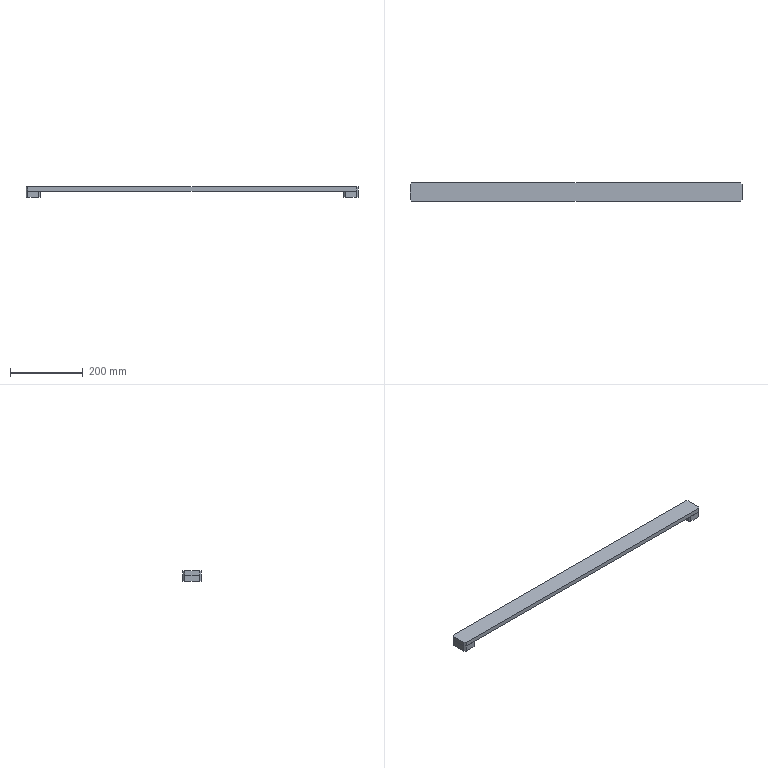Part | SolidWorks | features BaseBody 3 | 3 solids | 30 faces | box 913 x 50 x 29 mm | volume 613500 mm3 | plane 30
STEP:
#1=CARTESIAN_POINT('',(456.5,-20.,12.));
#2=VERTEX_POINT('',#1);
#3=CARTESIAN_POINT('',(456.5,20.,12.));
#4=VERTEX_POINT('',#3);
#5=CARTESIAN_POINT('',(456.5,25.,12.));
#6=DIRECTION('',(0.,1.,0.));
#7=VECTOR('',#6,1000.);
#8=LINE('',#5,#7);
#9=EDGE_CURVE('',#2,#4,#8,.T.);
#10=ORIENTED_EDGE('',*,*,#9,.F.);
#11=CARTESIAN_POINT('',(456.5,-20.,0.));
#12=VERTEX_POINT('',#11);
#13=CARTESIAN_POINT('',(456.5,-20.,12.));
#14=DIRECTION('',(0.,0.,-1.));
#15=VECTOR('',#14,1000.);
#16=LINE('',#13,#15);
#17=EDGE_CURVE('',#2,#12,#16,.T.);
#18=ORIENTED_EDGE('',*,*,#17,.T.);
#19=CARTESIAN_POINT('',(456.5,20.,0.));
#20=VERTEX_POINT('',#19);
#21=CARTESIAN_POINT('',(456.5,25.,0.));
#22=DIRECTION('',(0.,1.,0.));
#23=VECTOR('',#22,1000.);
#24=LINE('',#21,#23);
#25=EDGE_CURVE('',#12,#20,#24,.T.);
#26=ORIENTED_EDGE('',*,*,#25,.T.);
#27=CARTESIAN_POINT('',(456.5,20.,12.));
#28=DIRECTION('',(0.,0.,1.));
#29=VECTOR('',#28,1000.);
#30=LINE('',#27,#29);
#31=EDGE_CURVE('',#20,#4,#30,.T.);
#32=ORIENTED_EDGE('',*,*,#31,.T.);
#33=EDGE_LOOP('',(#10,#18,#26,#32));
#34=FACE_OUTER_BOUND('',#33,.T.);
#35=CARTESIAN_POINT('',(456.5,25.,12.));
#36=DIRECTION('',(-1.,0.,0.));
#37=DIRECTION('',(0.,0.,1.));
#38=AXIS2_PLACEMENT_3D('',#35,#36,#37);
#39=PLANE('',#38);
#40=ADVANCED_FACE('',(#34),#39,.F.);
#41=CARTESIAN_POINT('',(451.5,25.,0.));
#42=VERTEX_POINT('',#41);
#43=CARTESIAN_POINT('',(-451.5,25.,0.));
#44=VERTEX_POINT('',#43);
#45=CARTESIAN_POINT('',(-456.5,25.,0.));
#46=DIRECTION('',(-1.,0.,0.));
#47=VECTOR('',#46,1000.);
#48=LINE('',#45,#47);
#49=EDGE_CURVE('',#42,#44,#48,.T.);
#50=ORIENTED_EDGE('',*,*,#49,.T.);
#51=CARTESIAN_POINT('',(-451.5,25.,12.));
#52=VERTEX_POINT('',#51);
#53=CARTESIAN_POINT('',(-451.5,25.,12.));
#54=DIRECTION('',(0.,0.,1.));
#55=VECTOR('',#54,1000.);
#56=LINE('',#53,#55);
#57=EDGE_CURVE('',#44,#52,#56,.T.);
#58=ORIENTED_EDGE('',*,*,#57,.T.);
#59=CARTESIAN_POINT('',(451.5,25.,12.));
#60=VERTEX_POINT('',#59);
#61=CARTESIAN_POINT('',(-130.,25.,12.));
#62=DIRECTION('',(-1.,0.,0.));
#63=VECTOR('',#62,1000.);
#64=LINE('',#61,#63);
#65=EDGE_CURVE('',#60,#52,#64,.T.);
#66=ORIENTED_EDGE('',*,*,#65,.F.);
#67=CARTESIAN_POINT('',(451.5,25.,12.));
#68=DIRECTION('',(0.,0.,-1.));
#69=VECTOR('',#68,1000.);
#70=LINE('',#67,#69);
#71=EDGE_CURVE('',#60,#42,#70,.T.);
#72=ORIENTED_EDGE('',*,*,#71,.T.);
#73=EDGE_LOOP('',(#50,#58,#66,#72));
#74=FACE_OUTER_BOUND('',#73,.T.);
#75=CARTESIAN_POINT('',(-456.5,25.,12.));
#76=DIRECTION('',(0.,-1.,0.));
#77=DIRECTION('',(0.,0.,-1.));
#78=AXIS2_PLACEMENT_3D('',#75,#76,#77);
#79=PLANE('',#78);
#80=ADVANCED_FACE('',(#74),#79,.F.);
#81=CARTESIAN_POINT('',(-456.5,20.,12.));
#82=VERTEX_POINT('',#81);
#83=CARTESIAN_POINT('',(-456.5,-20.,12.));
#84=VERTEX_POINT('',#83);
#85=CARTESIAN_POINT('',(-456.5,25.,12.));
#86=DIRECTION('',(0.,-1.,0.));
#87=VECTOR('',#86,1000.);
#88=LINE('',#85,#87);
#89=EDGE_CURVE('',#82,#84,#88,.T.);
#90=ORIENTED_EDGE('',*,*,#89,.F.);
#91=CARTESIAN_POINT('',(-456.5,20.,0.));
#92=VERTEX_POINT('',#91);
#93=CARTESIAN_POINT('',(-456.5,20.,12.));
#94=DIRECTION('',(0.,0.,-1.));
#95=VECTOR('',#94,1000.);
#96=LINE('',#93,#95);
#97=EDGE_CURVE('',#82,#92,#96,.T.);
#98=ORIENTED_EDGE('',*,*,#97,.T.);
#99=CARTESIAN_POINT('',(-456.5,-20.,0.));
#100=VERTEX_POINT('',#99);
#101=CARTESIAN_POINT('',(-456.5,25.,0.));
#102=DIRECTION('',(0.,-1.,0.));
#103=VECTOR('',#102,1000.);
#104=LINE('',#101,#103);
#105=EDGE_CURVE('',#92,#100,#104,.T.);
#106=ORIENTED_EDGE('',*,*,#105,.T.);
#107=CARTESIAN_POINT('',(-456.5,-20.,12.));
#108=DIRECTION('',(0.,0.,1.));
#109=VECTOR('',#108,1000.);
#110=LINE('',#107,#109);
#111=EDGE_CURVE('',#100,#84,#110,.T.);
#112=ORIENTED_EDGE('',*,*,#111,.T.);
#113=EDGE_LOOP('',(#90,#98,#106,#112));
#114=FACE_OUTER_BOUND('',#113,.T.);
#115=CARTESIAN_POINT('',(-456.5,25.,12.));
#116=DIRECTION('',(1.,0.,0.));
#117=DIRECTION('',(0.,0.,-1.));
#118=AXIS2_PLACEMENT_3D('',#115,#116,#117);
#119=PLANE('',#118);
#120=ADVANCED_FACE('',(#114),#119,.F.);
#121=CARTESIAN_POINT('',(-451.5,-25.,12.));
#122=VERTEX_POINT('',#121);
#123=CARTESIAN_POINT('',(451.5,-25.,12.));
#124=VERTEX_POINT('',#123);
#125=CARTESIAN_POINT('',(-456.5,-25.,12.));
#126=DIRECTION('',(1.,0.,0.));
#127=VECTOR('',#126,1000.);
#128=LINE('',#125,#127);
#129=EDGE_CURVE('',#122,#124,#128,.T.);
#130=ORIENTED_EDGE('',*,*,#129,.F.);
#131=CARTESIAN_POINT('',(-451.5,-25.,0.));
#132=VERTEX_POINT('',#131);
#133=CARTESIAN_POINT('',(-451.5,-25.,12.));
#134=DIRECTION('',(0.,0.,-1.));
#135=VECTOR('',#134,1000.);
#136=LINE('',#133,#135);
#137=EDGE_CURVE('',#122,#132,#136,.T.);
#138=ORIENTED_EDGE('',*,*,#137,.T.);
#139=CARTESIAN_POINT('',(451.5,-25.,0.));
#140=VERTEX_POINT('',#139);
#141=CARTESIAN_POINT('',(-456.5,-25.,0.));
#142=DIRECTION('',(1.,0.,0.));
#143=VECTOR('',#142,1000.);
#144=LINE('',#141,#143);
#145=EDGE_CURVE('',#132,#140,#144,.T.);
#146=ORIENTED_EDGE('',*,*,#145,.T.);
#147=CARTESIAN_POINT('',(451.5,-25.,12.));
#148=DIRECTION('',(0.,0.,1.));
#149=VECTOR('',#148,1000.);
#150=LINE('',#147,#149);
#151=EDGE_CURVE('',#140,#124,#150,.T.);
#152=ORIENTED_EDGE('',*,*,#151,.T.);
#153=EDGE_LOOP('',(#130,#138,#146,#152));
#154=FACE_OUTER_BOUND('',#153,.T.);
#155=CARTESIAN_POINT('',(-456.5,-25.,12.));
#156=DIRECTION('',(0.,1.,0.));
#157=DIRECTION('',(0.,0.,1.));
#158=AXIS2_PLACEMENT_3D('',#155,#156,#157);
#159=PLANE('',#158);
#160=ADVANCED_FACE('',(#154),#159,.F.);
#161=ORIENTED_EDGE('',*,*,#65,.T.);
#162=CARTESIAN_POINT('',(-238.25,238.25,12.));
#163=DIRECTION('',(-0.7071,-0.7071,0.));
#164=VECTOR('',#163,1000.);
#165=LINE('',#162,#164);
#166=EDGE_CURVE('',#52,#82,#165,.T.);
#167=ORIENTED_EDGE('',*,*,#166,.T.);
#168=ORIENTED_EDGE('',*,*,#89,.T.);
#169=CARTESIAN_POINT('',(-238.25,-238.25,12.));
#170=DIRECTION('',(0.7071,-0.7071,0.));
#171=VECTOR('',#170,1000.);
#172=LINE('',#169,#171);
#173=EDGE_CURVE('',#84,#122,#172,.T.);
#174=ORIENTED_EDGE('',*,*,#173,.T.);
#175=ORIENTED_EDGE('',*,*,#129,.T.);
#176=CARTESIAN_POINT('',(238.25,-238.25,12.));
#177=DIRECTION('',(0.7071,0.7071,0.));
#178=VECTOR('',#177,1000.);
#179=LINE('',#176,#178);
#180=EDGE_CURVE('',#124,#2,#179,.T.);
#181=ORIENTED_EDGE('',*,*,#180,.T.);
#182=ORIENTED_EDGE('',*,*,#9,.T.);
#183=CARTESIAN_POINT('',(238.25,238.25,12.));
#184=DIRECTION('',(-0.7071,0.7071,0.));
#185=VECTOR('',#184,1000.);
#186=LINE('',#183,#185);
#187=EDGE_CURVE('',#4,#60,#186,.T.);
#188=ORIENTED_EDGE('',*,*,#187,.T.);
#189=EDGE_LOOP('',(#161,#167,#168,#174,#175,#181,#182,#188));
#190=FACE_OUTER_BOUND('',#189,.T.);
#191=CARTESIAN_POINT('',(0.,0.,12.));
#192=DIRECTION('',(0.,0.,1.));
#193=DIRECTION('',(1.,0.,0.));
#194=AXIS2_PLACEMENT_3D('',#191,#192,#193);
#195=PLANE('',#194);
#196=ADVANCED_FACE('',(#190),#195,.T.);
#197=ORIENTED_EDGE('',*,*,#105,.F.);
#198=CARTESIAN_POINT('',(-456.5,20.,0.));
#199=DIRECTION('',(0.7071,0.7071,0.));
#200=VECTOR('',#199,1000.);
#201=LINE('',#198,#200);
#202=EDGE_CURVE('',#92,#44,#201,.T.);
#203=ORIENTED_EDGE('',*,*,#202,.T.);
#204=ORIENTED_EDGE('',*,*,#49,.F.);
#205=CARTESIAN_POINT('',(451.5,25.,0.));
#206=DIRECTION('',(0.7071,-0.7071,0.));
#207=VECTOR('',#206,1000.);
#208=LINE('',#205,#207);
#209=EDGE_CURVE('',#42,#20,#208,.T.);
#210=ORIENTED_EDGE('',*,*,#209,.T.);
#211=ORIENTED_EDGE('',*,*,#25,.F.);
#212=CARTESIAN_POINT('',(456.5,-20.,0.));
#213=DIRECTION('',(-0.7071,-0.7071,0.));
#214=VECTOR('',#213,1000.);
#215=LINE('',#212,#214);
#216=EDGE_CURVE('',#12,#140,#215,.T.);
#217=ORIENTED_EDGE('',*,*,#216,.T.);
#218=ORIENTED_EDGE('',*,*,#145,.F.);
#219=CARTESIAN_POINT('',(-451.5,-25.,0.));
#220=DIRECTION('',(-0.7071,0.7071,0.));
#221=VECTOR('',#220,1000.);
#222=LINE('',#219,#221);
#223=EDGE_CURVE('',#132,#100,#222,.T.);
#224=ORIENTED_EDGE('',*,*,#223,.T.);
#225=EDGE_LOOP('',(#197,#203,#204,#210,#211,#217,#218,#224));
#226=FACE_OUTER_BOUND('',#225,.T.);
#227=CARTESIAN_POINT('',(0.,0.,0.));
#228=DIRECTION('',(0.,0.,1.));
#229=DIRECTION('',(1.,0.,0.));
#230=AXIS2_PLACEMENT_3D('',#227,#228,#229);
#231=PLANE('',#230);
#232=ADVANCED_FACE('',(#226),#231,.F.);
#233=ORIENTED_EDGE('',*,*,#166,.F.);
#234=ORIENTED_EDGE('',*,*,#57,.F.);
#235=ORIENTED_EDGE('',*,*,#202,.F.);
#236=ORIENTED_EDGE('',*,*,#97,.F.);
#237=EDGE_LOOP('',(#233,#234,#235,#236));
#238=FACE_OUTER_BOUND('',#237,.T.);
#239=CARTESIAN_POINT('',(-456.5,20.,12.));
#240=DIRECTION('',(0.7071,-0.7071,0.));
#241=DIRECTION('',(0.,0.,-1.));
#242=AXIS2_PLACEMENT_3D('',#239,#240,#241);
#243=PLANE('',#242);
#244=ADVANCED_FACE('',(#238),#243,.F.);
#245=ORIENTED_EDGE('',*,*,#173,.F.);
#246=ORIENTED_EDGE('',*,*,#111,.F.);
#247=ORIENTED_EDGE('',*,*,#223,.F.);
#248=ORIENTED_EDGE('',*,*,#137,.F.);
#249=EDGE_LOOP('',(#245,#246,#247,#248));
#250=FACE_OUTER_BOUND('',#249,.T.);
#251=CARTESIAN_POINT('',(-451.5,-25.,12.));
#252=DIRECTION('',(0.7071,0.7071,0.));
#253=DIRECTION('',(0.,0.,-1.));
#254=AXIS2_PLACEMENT_3D('',#251,#252,#253);
#255=PLANE('',#254);
#256=ADVANCED_FACE('',(#250),#255,.F.);
#257=ORIENTED_EDGE('',*,*,#180,.F.);
#258=ORIENTED_EDGE('',*,*,#151,.F.);
#259=ORIENTED_EDGE('',*,*,#216,.F.);
#260=ORIENTED_EDGE('',*,*,#17,.F.);
#261=EDGE_LOOP('',(#257,#258,#259,#260));
#262=FACE_OUTER_BOUND('',#261,.T.);
#263=CARTESIAN_POINT('',(456.5,-20.,12.));
#264=DIRECTION('',(-0.7071,0.7071,0.));
#265=DIRECTION('',(0.,0.,-1.));
#266=AXIS2_PLACEMENT_3D('',#263,#264,#265);
#267=PLANE('',#266);
#268=ADVANCED_FACE('',(#262),#267,.F.);
#269=ORIENTED_EDGE('',*,*,#187,.F.);
#270=ORIENTED_EDGE('',*,*,#31,.F.);
#271=ORIENTED_EDGE('',*,*,#209,.F.);
#272=ORIENTED_EDGE('',*,*,#71,.F.);
#273=EDGE_LOOP('',(#269,#270,#271,#272));
#274=FACE_OUTER_BOUND('',#273,.T.);
#275=CARTESIAN_POINT('',(451.5,25.,12.));
#276=DIRECTION('',(-0.7071,-0.7071,0.));
#277=DIRECTION('',(0.,0.,-1.));
#278=AXIS2_PLACEMENT_3D('',#275,#276,#277);
#279=PLANE('',#278);
#280=ADVANCED_FACE('',(#274),#279,.F.);
#281=CLOSED_SHELL('',(#40,#80,#120,#160,#196,#232,#244,#256,#268,#280));
#282=MANIFOLD_SOLID_BREP('',#281);
#283=CARTESIAN_POINT('',(-456.5,-20.,0.));
#284=VERTEX_POINT('',#283);
#285=CARTESIAN_POINT('',(-451.5,-25.,0.));
#286=VERTEX_POINT('',#285);
#287=CARTESIAN_POINT('',(-456.5,-20.,0.));
#288=DIRECTION('',(0.7071,-0.7071,0.));
#289=VECTOR('',#288,1000.);
#290=LINE('',#287,#289);
#291=EDGE_CURVE('',#284,#286,#290,.T.);
#292=ORIENTED_EDGE('',*,*,#291,.F.);
#293=CARTESIAN_POINT('',(-456.5,-20.,-17.));
#294=VERTEX_POINT('',#293);
#295=CARTESIAN_POINT('',(-456.5,-20.,-17.));
#296=DIRECTION('',(0.,0.,1.));
#297=VECTOR('',#296,1000.);
#298=LINE('',#295,#297);
#299=EDGE_CURVE('',#294,#284,#298,.T.);
#300=ORIENTED_EDGE('',*,*,#299,.F.);
#301=CARTESIAN_POINT('',(-451.5,-25.,-17.));
#302=VERTEX_POINT('',#301);
#303=CARTESIAN_POINT('',(-456.5,-20.,-17.));
#304=DIRECTION('',(0.7071,-0.7071,0.));
#305=VECTOR('',#304,1000.);
#306=LINE('',#303,#305);
#307=EDGE_CURVE('',#294,#302,#306,.T.);
#308=ORIENTED_EDGE('',*,*,#307,.T.);
#309=CARTESIAN_POINT('',(-451.5,-25.,-17.));
#310=DIRECTION('',(0.,0.,1.));
#311=VECTOR('',#310,1000.);
#312=LINE('',#309,#311);
#313=EDGE_CURVE('',#302,#286,#312,.T.);
#314=ORIENTED_EDGE('',*,*,#313,.T.);
#315=EDGE_LOOP('',(#292,#300,#308,#314));
#316=FACE_OUTER_BOUND('',#315,.T.);
#317=CARTESIAN_POINT('',(-456.5,-20.,-17.));
#318=DIRECTION('',(-0.7071,-0.7071,0.));
#319=DIRECTION('',(0.7071,-0.7071,0.));
#320=AXIS2_PLACEMENT_3D('',#317,#318,#319);
#321=PLANE('',#320);
#322=ADVANCED_FACE('',(#316),#321,.T.);
#323=CARTESIAN_POINT('',(-456.5,20.,0.));
#324=VERTEX_POINT('',#323);
#325=CARTESIAN_POINT('',(-456.5,-20.,0.));
#326=DIRECTION('',(0.,-1.,0.));
#327=VECTOR('',#326,1000.);
#328=LINE('',#325,#327);
#329=EDGE_CURVE('',#324,#284,#328,.T.);
#330=ORIENTED_EDGE('',*,*,#329,.F.);
#331=CARTESIAN_POINT('',(-456.5,20.,-17.));
#332=VERTEX_POINT('',#331);
#333=CARTESIAN_POINT('',(-456.5,20.,-17.));
#334=DIRECTION('',(0.,0.,1.));
#335=VECTOR('',#334,1000.);
#336=LINE('',#333,#335);
#337=EDGE_CURVE('',#332,#324,#336,.T.);
#338=ORIENTED_EDGE('',*,*,#337,.F.);
#339=CARTESIAN_POINT('',(-456.5,-20.,-17.));
#340=DIRECTION('',(0.,-1.,0.));
#341=VECTOR('',#340,1000.);
#342=LINE('',#339,#341);
#343=EDGE_CURVE('',#332,#294,#342,.T.);
#344=ORIENTED_EDGE('',*,*,#343,.T.);
#345=ORIENTED_EDGE('',*,*,#299,.T.);
#346=EDGE_LOOP('',(#330,#338,#344,#345));
#347=FACE_OUTER_BOUND('',#346,.T.);
#348=CARTESIAN_POINT('',(-456.5,-20.,-17.));
#349=DIRECTION('',(-1.,0.,0.));
#350=DIRECTION('',(0.,0.,1.));
#351=AXIS2_PLACEMENT_3D('',#348,#349,#350);
#352=PLANE('',#351);
#353=ADVANCED_FACE('',(#347),#352,.T.);
#354=CARTESIAN_POINT('',(-451.5,25.,0.));
#355=VERTEX_POINT('',#354);
#356=CARTESIAN_POINT('',(-456.5,20.,0.));
#357=DIRECTION('',(-0.7071,-0.7071,0.));
#358=VECTOR('',#357,1000.);
#359=LINE('',#356,#358);
#360=EDGE_CURVE('',#355,#324,#359,.T.);
#361=ORIENTED_EDGE('',*,*,#360,.F.);
#362=CARTESIAN_POINT('',(-451.5,25.,-17.));
#363=VERTEX_POINT('',#362);
#364=CARTESIAN_POINT('',(-451.5,25.,-17.));
#365=DIRECTION('',(0.,0.,1.));
#366=VECTOR('',#365,1000.);
#367=LINE('',#364,#366);
#368=EDGE_CURVE('',#363,#355,#367,.T.);
#369=ORIENTED_EDGE('',*,*,#368,.F.);
#370=CARTESIAN_POINT('',(-456.5,20.,-17.));
#371=DIRECTION('',(-0.7071,-0.7071,0.));
#372=VECTOR('',#371,1000.);
#373=LINE('',#370,#372);
#374=EDGE_CURVE('',#363,#332,#373,.T.);
#375=ORIENTED_EDGE('',*,*,#374,.T.);
#376=ORIENTED_EDGE('',*,*,#337,.T.);
#377=EDGE_LOOP('',(#361,#369,#375,#376));
#378=FACE_OUTER_BOUND('',#377,.T.);
#379=CARTESIAN_POINT('',(-456.5,20.,-17.));
#380=DIRECTION('',(-0.7071,0.7071,0.));
#381=DIRECTION('',(-0.7071,-0.7071,0.));
#382=AXIS2_PLACEMENT_3D('',#379,#380,#381);
#383=PLANE('',#382);
#384=ADVANCED_FACE('',(#378),#383,.T.);
#385=CARTESIAN_POINT('',(-421.5,25.,0.));
#386=VERTEX_POINT('',#385);
#387=CARTESIAN_POINT('',(-451.5,25.,0.));
#388=DIRECTION('',(-1.,0.,0.));
#389=VECTOR('',#388,1000.);
#390=LINE('',#387,#389);
#391=EDGE_CURVE('',#386,#355,#390,.T.);
#392=ORIENTED_EDGE('',*,*,#391,.F.);
#393=CARTESIAN_POINT('',(-421.5,25.,-17.));
#394=VERTEX_POINT('',#393);
#395=CARTESIAN_POINT('',(-421.5,25.,-17.));
#396=DIRECTION('',(0.,0.,1.));
#397=VECTOR('',#396,1000.);
#398=LINE('',#395,#397);
#399=EDGE_CURVE('',#394,#386,#398,.T.);
#400=ORIENTED_EDGE('',*,*,#399,.F.);
#401=CARTESIAN_POINT('',(-451.5,25.,-17.));
#402=DIRECTION('',(-1.,0.,0.));
#403=VECTOR('',#402,1000.);
#404=LINE('',#401,#403);
#405=EDGE_CURVE('',#394,#363,#404,.T.);
#406=ORIENTED_EDGE('',*,*,#405,.T.);
#407=ORIENTED_EDGE('',*,*,#368,.T.);
#408=EDGE_LOOP('',(#392,#400,#406,#407));
#409=FACE_OUTER_BOUND('',#408,.T.);
#410=CARTESIAN_POINT('',(-451.5,25.,-17.));
#411=DIRECTION('',(0.,1.,0.));
#412=DIRECTION('',(0.,0.,1.));
#413=AXIS2_PLACEMENT_3D('',#410,#411,#412);
#414=PLANE('',#413);
#415=ADVANCED_FACE('',(#409),#414,.T.);
#416=CARTESIAN_POINT('',(-416.5,20.,0.));
#417=VERTEX_POINT('',#416);
#418=CARTESIAN_POINT('',(-421.5,25.,0.));
#419=DIRECTION('',(-0.7071,0.7071,0.));
#420=VECTOR('',#419,1000.);
#421=LINE('',#418,#420);
#422=EDGE_CURVE('',#417,#386,#421,.T.);
#423=ORIENTED_EDGE('',*,*,#422,.F.);
#424=CARTESIAN_POINT('',(-416.5,20.,-17.));
#425=VERTEX_POINT('',#424);
#426=CARTESIAN_POINT('',(-416.5,20.,-17.));
#427=DIRECTION('',(0.,0.,1.));
#428=VECTOR('',#427,1000.);
#429=LINE('',#426,#428);
#430=EDGE_CURVE('',#425,#417,#429,.T.);
#431=ORIENTED_EDGE('',*,*,#430,.F.);
#432=CARTESIAN_POINT('',(-421.5,25.,-17.));
#433=DIRECTION('',(-0.7071,0.7071,0.));
#434=VECTOR('',#433,1000.);
#435=LINE('',#432,#434);
#436=EDGE_CURVE('',#425,#394,#435,.T.);
#437=ORIENTED_EDGE('',*,*,#436,.T.);
#438=ORIENTED_EDGE('',*,*,#399,.T.);
#439=EDGE_LOOP('',(#423,#431,#437,#438));
#440=FACE_OUTER_BOUND('',#439,.T.);
#441=CARTESIAN_POINT('',(-421.5,25.,-17.));
#442=DIRECTION('',(0.7071,0.7071,0.));
#443=DIRECTION('',(-0.7071,0.7071,0.));
#444=AXIS2_PLACEMENT_3D('',#441,#442,#443);
#445=PLANE('',#444);
#446=ADVANCED_FACE('',(#440),#445,.T.);
#447=CARTESIAN_POINT('',(-416.5,-20.,0.));
#448=VERTEX_POINT('',#447);
#449=CARTESIAN_POINT('',(-416.5,-20.,0.));
#450=DIRECTION('',(0.,1.,0.));
#451=VECTOR('',#450,1000.);
#452=LINE('',#449,#451);
#453=EDGE_CURVE('',#448,#417,#452,.T.);
#454=ORIENTED_EDGE('',*,*,#453,.F.);
#455=CARTESIAN_POINT('',(-416.5,-20.,-17.));
#456=VERTEX_POINT('',#455);
#457=CARTESIAN_POINT('',(-416.5,-20.,-17.));
#458=DIRECTION('',(0.,0.,1.));
#459=VECTOR('',#458,1000.);
#460=LINE('',#457,#459);
#461=EDGE_CURVE('',#456,#448,#460,.T.);
#462=ORIENTED_EDGE('',*,*,#461,.F.);
#463=CARTESIAN_POINT('',(-416.5,-20.,-17.));
#464=DIRECTION('',(0.,1.,0.));
#465=VECTOR('',#464,1000.);
#466=LINE('',#463,#465);
#467=EDGE_CURVE('',#456,#425,#466,.T.);
#468=ORIENTED_EDGE('',*,*,#467,.T.);
#469=ORIENTED_EDGE('',*,*,#430,.T.);
#470=EDGE_LOOP('',(#454,#462,#468,#469));
#471=FACE_OUTER_BOUND('',#470,.T.);
#472=CARTESIAN_POINT('',(-416.5,-20.,-17.));
#473=DIRECTION('',(1.,0.,0.));
#474=DIRECTION('',(0.,0.,-1.));
#475=AXIS2_PLACEMENT_3D('',#472,#473,#474);
#476=PLANE('',#475);
#477=ADVANCED_FACE('',(#471),#476,.T.);
#478=CARTESIAN_POINT('',(-421.5,-25.,0.));
#479=VERTEX_POINT('',#478);
#480=CARTESIAN_POINT('',(-421.5,-25.,0.));
#481=DIRECTION('',(0.7071,0.7071,0.));
#482=VECTOR('',#481,1000.);
#483=LINE('',#480,#482);
#484=EDGE_CURVE('',#479,#448,#483,.T.);
#485=ORIENTED_EDGE('',*,*,#484,.F.);
#486=CARTESIAN_POINT('',(-421.5,-25.,-17.));
#487=VERTEX_POINT('',#486);
#488=CARTESIAN_POINT('',(-421.5,-25.,-17.));
#489=DIRECTION('',(0.,0.,1.));
#490=VECTOR('',#489,1000.);
#491=LINE('',#488,#490);
#492=EDGE_CURVE('',#487,#479,#491,.T.);
#493=ORIENTED_EDGE('',*,*,#492,.F.);
#494=CARTESIAN_POINT('',(-421.5,-25.,-17.));
#495=DIRECTION('',(0.7071,0.7071,0.));
#496=VECTOR('',#495,1000.);
#497=LINE('',#494,#496);
#498=EDGE_CURVE('',#487,#456,#497,.T.);
#499=ORIENTED_EDGE('',*,*,#498,.T.);
#500=ORIENTED_EDGE('',*,*,#461,.T.);
#501=EDGE_LOOP('',(#485,#493,#499,#500));
#502=FACE_OUTER_BOUND('',#501,.T.);
#503=CARTESIAN_POINT('',(-421.5,-25.,-17.));
#504=DIRECTION('',(0.7071,-0.7071,0.));
#505=DIRECTION('',(0.7071,0.7071,0.));
#506=AXIS2_PLACEMENT_3D('',#503,#504,#505);
#507=PLANE('',#506);
#508=ADVANCED_FACE('',(#502),#507,.T.);
#509=CARTESIAN_POINT('',(-451.5,-25.,0.));
#510=DIRECTION('',(1.,0.,0.));
#511=VECTOR('',#510,1000.);
#512=LINE('',#509,#511);
#513=EDGE_CURVE('',#286,#479,#512,.T.);
#514=ORIENTED_EDGE('',*,*,#513,.F.);
#515=ORIENTED_EDGE('',*,*,#313,.F.);
#516=CARTESIAN_POINT('',(-451.5,-25.,-17.));
#517=DIRECTION('',(1.,0.,0.));
#518=VECTOR('',#517,1000.);
#519=LINE('',#516,#518);
#520=EDGE_CURVE('',#302,#487,#519,.T.);
#521=ORIENTED_EDGE('',*,*,#520,.T.);
#522=ORIENTED_EDGE('',*,*,#492,.T.);
#523=EDGE_LOOP('',(#514,#515,#521,#522));
#524=FACE_OUTER_BOUND('',#523,.T.);
#525=CARTESIAN_POINT('',(-451.5,-25.,-17.));
#526=DIRECTION('',(0.,-1.,0.));
#527=DIRECTION('',(0.,0.,-1.));
#528=AXIS2_PLACEMENT_3D('',#525,#526,#527);
#529=PLANE('',#528);
#530=ADVANCED_FACE('',(#524),#529,.T.);
#531=ORIENTED_EDGE('',*,*,#307,.F.);
#532=ORIENTED_EDGE('',*,*,#343,.F.);
#533=ORIENTED_EDGE('',*,*,#374,.F.);
#534=ORIENTED_EDGE('',*,*,#405,.F.);
#535=ORIENTED_EDGE('',*,*,#436,.F.);
#536=ORIENTED_EDGE('',*,*,#467,.F.);
#537=ORIENTED_EDGE('',*,*,#498,.F.);
#538=ORIENTED_EDGE('',*,*,#520,.F.);
#539=EDGE_LOOP('',(#531,#532,#533,#534,#535,#536,#537,#538));
#540=FACE_OUTER_BOUND('',#539,.T.);
#541=CARTESIAN_POINT('',(0.,0.,-17.));
#542=DIRECTION('',(0.,0.,1.));
#543=DIRECTION('',(1.,0.,0.));
#544=AXIS2_PLACEMENT_3D('',#541,#542,#543);
#545=PLANE('',#544);
#546=ADVANCED_FACE('',(#540),#545,.F.);
#547=ORIENTED_EDGE('',*,*,#291,.T.);
#548=ORIENTED_EDGE('',*,*,#513,.T.);
#549=ORIENTED_EDGE('',*,*,#484,.T.);
#550=ORIENTED_EDGE('',*,*,#453,.T.);
#551=ORIENTED_EDGE('',*,*,#422,.T.);
#552=ORIENTED_EDGE('',*,*,#391,.T.);
#553=ORIENTED_EDGE('',*,*,#360,.T.);
#554=ORIENTED_EDGE('',*,*,#329,.T.);
#555=EDGE_LOOP('',(#547,#548,#549,#550,#551,#552,#553,#554));
#556=FACE_OUTER_BOUND('',#555,.T.);
#557=CARTESIAN_POINT('',(0.,0.,0.));
#558=DIRECTION('',(0.,0.,1.));
#559=DIRECTION('',(1.,0.,0.));
#560=AXIS2_PLACEMENT_3D('',#557,#558,#559);
#561=PLANE('',#560);
#562=ADVANCED_FACE('',(#556),#561,.T.);
#563=CLOSED_SHELL('',(#322,#353,#384,#415,#446,#477,#508,#530,#546,#562));
#564=MANIFOLD_SOLID_BREP('',#563);
#565=CARTESIAN_POINT('',(456.5,20.,0.));
#566=VERTEX_POINT('',#565);
#567=CARTESIAN_POINT('',(451.5,25.,0.));
#568=VERTEX_POINT('',#567);
#569=CARTESIAN_POINT('',(456.5,20.,0.));
#570=DIRECTION('',(-0.7071,0.7071,0.));
#571=VECTOR('',#570,1000.);
#572=LINE('',#569,#571);
#573=EDGE_CURVE('',#566,#568,#572,.T.);
#574=ORIENTED_EDGE('',*,*,#573,.F.);
#575=CARTESIAN_POINT('',(456.5,20.,-17.));
#576=VERTEX_POINT('',#575);
#577=CARTESIAN_POINT('',(456.5,20.,-17.));
#578=DIRECTION('',(0.,0.,1.));
#579=VECTOR('',#578,1000.);
#580=LINE('',#577,#579);
#581=EDGE_CURVE('',#576,#566,#580,.T.);
#582=ORIENTED_EDGE('',*,*,#581,.F.);
#583=CARTESIAN_POINT('',(451.5,25.,-17.));
#584=VERTEX_POINT('',#583);
#585=CARTESIAN_POINT('',(456.5,20.,-17.));
#586=DIRECTION('',(-0.7071,0.7071,0.));
#587=VECTOR('',#586,1000.);
#588=LINE('',#585,#587);
#589=EDGE_CURVE('',#576,#584,#588,.T.);
#590=ORIENTED_EDGE('',*,*,#589,.T.);
#591=CARTESIAN_POINT('',(451.5,25.,-17.));
#592=DIRECTION('',(0.,0.,1.));
#593=VECTOR('',#592,1000.);
#594=LINE('',#591,#593);
#595=EDGE_CURVE('',#584,#568,#594,.T.);
#596=ORIENTED_EDGE('',*,*,#595,.T.);
#597=EDGE_LOOP('',(#574,#582,#590,#596));
#598=FACE_OUTER_BOUND('',#597,.T.);
#599=CARTESIAN_POINT('',(456.5,20.,-17.));
#600=DIRECTION('',(0.7071,0.7071,0.));
#601=DIRECTION('',(-0.7071,0.7071,0.));
#602=AXIS2_PLACEMENT_3D('',#599,#600,#601);
#603=PLANE('',#602);
#604=ADVANCED_FACE('',(#598),#603,.T.);
#605=CARTESIAN_POINT('',(456.5,-20.,0.));
#606=VERTEX_POINT('',#605);
#607=CARTESIAN_POINT('',(456.5,-20.,0.));
#608=DIRECTION('',(0.,1.,0.));
#609=VECTOR('',#608,1000.);
#610=LINE('',#607,#609);
#611=EDGE_CURVE('',#606,#566,#610,.T.);
#612=ORIENTED_EDGE('',*,*,#611,.F.);
#613=CARTESIAN_POINT('',(456.5,-20.,-17.));
#614=VERTEX_POINT('',#613);
#615=CARTESIAN_POINT('',(456.5,-20.,-17.));
#616=DIRECTION('',(0.,0.,1.));
#617=VECTOR('',#616,1000.);
#618=LINE('',#615,#617);
#619=EDGE_CURVE('',#614,#606,#618,.T.);
#620=ORIENTED_EDGE('',*,*,#619,.F.);
#621=CARTESIAN_POINT('',(456.5,-20.,-17.));
#622=DIRECTION('',(0.,1.,0.));
#623=VECTOR('',#622,1000.);
#624=LINE('',#621,#623);
#625=EDGE_CURVE('',#614,#576,#624,.T.);
#626=ORIENTED_EDGE('',*,*,#625,.T.);
#627=ORIENTED_EDGE('',*,*,#581,.T.);
#628=EDGE_LOOP('',(#612,#620,#626,#627));
#629=FACE_OUTER_BOUND('',#628,.T.);
#630=CARTESIAN_POINT('',(456.5,-20.,-17.));
#631=DIRECTION('',(1.,0.,0.));
#632=DIRECTION('',(0.,0.,-1.));
#633=AXIS2_PLACEMENT_3D('',#630,#631,#632);
#634=PLANE('',#633);
#635=ADVANCED_FACE('',(#629),#634,.T.);
#636=CARTESIAN_POINT('',(451.5,-25.,0.));
#637=VERTEX_POINT('',#636);
#638=CARTESIAN_POINT('',(456.5,-20.,0.));
#639=DIRECTION('',(0.7071,0.7071,0.));
#640=VECTOR('',#639,1000.);
#641=LINE('',#638,#640);
#642=EDGE_CURVE('',#637,#606,#641,.T.);
#643=ORIENTED_EDGE('',*,*,#642,.F.);
#644=CARTESIAN_POINT('',(451.5,-25.,-17.));
#645=VERTEX_POINT('',#644);
#646=CARTESIAN_POINT('',(451.5,-25.,-17.));
#647=DIRECTION('',(0.,0.,1.));
#648=VECTOR('',#647,1000.);
#649=LINE('',#646,#648);
#650=EDGE_CURVE('',#645,#637,#649,.T.);
#651=ORIENTED_EDGE('',*,*,#650,.F.);
#652=CARTESIAN_POINT('',(456.5,-20.,-17.));
#653=DIRECTION('',(0.7071,0.7071,0.));
#654=VECTOR('',#653,1000.);
#655=LINE('',#652,#654);
#656=EDGE_CURVE('',#645,#614,#655,.T.);
#657=ORIENTED_EDGE('',*,*,#656,.T.);
#658=ORIENTED_EDGE('',*,*,#619,.T.);
#659=EDGE_LOOP('',(#643,#651,#657,#658));
#660=FACE_OUTER_BOUND('',#659,.T.);
#661=CARTESIAN_POINT('',(456.5,-20.,-17.));
#662=DIRECTION('',(0.7071,-0.7071,0.));
#663=DIRECTION('',(0.7071,0.7071,0.));
#664=AXIS2_PLACEMENT_3D('',#661,#662,#663);
#665=PLANE('',#664);
#666=ADVANCED_FACE('',(#660),#665,.T.);
#667=CARTESIAN_POINT('',(421.5,-25.,0.));
#668=VERTEX_POINT('',#667);
#669=CARTESIAN_POINT('',(451.5,-25.,0.));
#670=DIRECTION('',(1.,0.,0.));
#671=VECTOR('',#670,1000.);
#672=LINE('',#669,#671);
#673=EDGE_CURVE('',#668,#637,#672,.T.);
#674=ORIENTED_EDGE('',*,*,#673,.F.);
#675=CARTESIAN_POINT('',(421.5,-25.,-17.));
#676=VERTEX_POINT('',#675);
#677=CARTESIAN_POINT('',(421.5,-25.,-17.));
#678=DIRECTION('',(0.,0.,1.));
#679=VECTOR('',#678,1000.);
#680=LINE('',#677,#679);
#681=EDGE_CURVE('',#676,#668,#680,.T.);
#682=ORIENTED_EDGE('',*,*,#681,.F.);
#683=CARTESIAN_POINT('',(451.5,-25.,-17.));
#684=DIRECTION('',(1.,0.,0.));
#685=VECTOR('',#684,1000.);
#686=LINE('',#683,#685);
#687=EDGE_CURVE('',#676,#645,#686,.T.);
#688=ORIENTED_EDGE('',*,*,#687,.T.);
#689=ORIENTED_EDGE('',*,*,#650,.T.);
#690=EDGE_LOOP('',(#674,#682,#688,#689));
#691=FACE_OUTER_BOUND('',#690,.T.);
#692=CARTESIAN_POINT('',(451.5,-25.,-17.));
#693=DIRECTION('',(0.,-1.,0.));
#694=DIRECTION('',(0.,0.,-1.));
#695=AXIS2_PLACEMENT_3D('',#692,#693,#694);
#696=PLANE('',#695);
#697=ADVANCED_FACE('',(#691),#696,.T.);
#698=CARTESIAN_POINT('',(416.5,-20.,0.));
#699=VERTEX_POINT('',#698);
#700=CARTESIAN_POINT('',(421.5,-25.,0.));
#701=DIRECTION('',(0.7071,-0.7071,0.));
#702=VECTOR('',#701,1000.);
#703=LINE('',#700,#702);
#704=EDGE_CURVE('',#699,#668,#703,.T.);
#705=ORIENTED_EDGE('',*,*,#704,.F.);
#706=CARTESIAN_POINT('',(416.5,-20.,-17.));
#707=VERTEX_POINT('',#706);
#708=CARTESIAN_POINT('',(416.5,-20.,-17.));
#709=DIRECTION('',(0.,0.,1.));
#710=VECTOR('',#709,1000.);
#711=LINE('',#708,#710);
#712=EDGE_CURVE('',#707,#699,#711,.T.);
#713=ORIENTED_EDGE('',*,*,#712,.F.);
#714=CARTESIAN_POINT('',(421.5,-25.,-17.));
#715=DIRECTION('',(0.7071,-0.7071,0.));
#716=VECTOR('',#715,1000.);
#717=LINE('',#714,#716);
#718=EDGE_CURVE('',#707,#676,#717,.T.);
#719=ORIENTED_EDGE('',*,*,#718,.T.);
#720=ORIENTED_EDGE('',*,*,#681,.T.);
#721=EDGE_LOOP('',(#705,#713,#719,#720));
#722=FACE_OUTER_BOUND('',#721,.T.);
#723=CARTESIAN_POINT('',(421.5,-25.,-17.));
#724=DIRECTION('',(-0.7071,-0.7071,0.));
#725=DIRECTION('',(0.7071,-0.7071,0.));
#726=AXIS2_PLACEMENT_3D('',#723,#724,#725);
#727=PLANE('',#726);
#728=ADVANCED_FACE('',(#722),#727,.T.);
#729=CARTESIAN_POINT('',(416.5,20.,0.));
#730=VERTEX_POINT('',#729);
#731=CARTESIAN_POINT('',(416.5,-20.,0.));
#732=DIRECTION('',(0.,-1.,0.));
#733=VECTOR('',#732,1000.);
#734=LINE('',#731,#733);
#735=EDGE_CURVE('',#730,#699,#734,.T.);
#736=ORIENTED_EDGE('',*,*,#735,.F.);
#737=CARTESIAN_POINT('',(416.5,20.,-17.));
#738=VERTEX_POINT('',#737);
#739=CARTESIAN_POINT('',(416.5,20.,-17.));
#740=DIRECTION('',(0.,0.,1.));
#741=VECTOR('',#740,1000.);
#742=LINE('',#739,#741);
#743=EDGE_CURVE('',#738,#730,#742,.T.);
#744=ORIENTED_EDGE('',*,*,#743,.F.);
#745=CARTESIAN_POINT('',(416.5,-20.,-17.));
#746=DIRECTION('',(0.,-1.,0.));
#747=VECTOR('',#746,1000.);
#748=LINE('',#745,#747);
#749=EDGE_CURVE('',#738,#707,#748,.T.);
#750=ORIENTED_EDGE('',*,*,#749,.T.);
#751=ORIENTED_EDGE('',*,*,#712,.T.);
#752=EDGE_LOOP('',(#736,#744,#750,#751));
#753=FACE_OUTER_BOUND('',#752,.T.);
#754=CARTESIAN_POINT('',(416.5,-20.,-17.));
#755=DIRECTION('',(-1.,0.,0.));
#756=DIRECTION('',(0.,-1.,0.));
#757=AXIS2_PLACEMENT_3D('',#754,#755,#756);
#758=PLANE('',#757);
#759=ADVANCED_FACE('',(#753),#758,.T.);
#760=CARTESIAN_POINT('',(421.5,25.,0.));
#761=VERTEX_POINT('',#760);
#762=CARTESIAN_POINT('',(421.5,25.,0.));
#763=DIRECTION('',(-0.7071,-0.7071,0.));
#764=VECTOR('',#763,1000.);
#765=LINE('',#762,#764);
#766=EDGE_CURVE('',#761,#730,#765,.T.);
#767=ORIENTED_EDGE('',*,*,#766,.F.);
#768=CARTESIAN_POINT('',(421.5,25.,-17.));
#769=VERTEX_POINT('',#768);
#770=CARTESIAN_POINT('',(421.5,25.,-17.));
#771=DIRECTION('',(0.,0.,1.));
#772=VECTOR('',#771,1000.);
#773=LINE('',#770,#772);
#774=EDGE_CURVE('',#769,#761,#773,.T.);
#775=ORIENTED_EDGE('',*,*,#774,.F.);
#776=CARTESIAN_POINT('',(421.5,25.,-17.));
#777=DIRECTION('',(-0.7071,-0.7071,0.));
#778=VECTOR('',#777,1000.);
#779=LINE('',#776,#778);
#780=EDGE_CURVE('',#769,#738,#779,.T.);
#781=ORIENTED_EDGE('',*,*,#780,.T.);
#782=ORIENTED_EDGE('',*,*,#743,.T.);
#783=EDGE_LOOP('',(#767,#775,#781,#782));
#784=FACE_OUTER_BOUND('',#783,.T.);
#785=CARTESIAN_POINT('',(421.5,25.,-17.));
#786=DIRECTION('',(-0.7071,0.7071,0.));
#787=DIRECTION('',(-0.7071,-0.7071,0.));
#788=AXIS2_PLACEMENT_3D('',#785,#786,#787);
#789=PLANE('',#788);
#790=ADVANCED_FACE('',(#784),#789,.T.);
#791=CARTESIAN_POINT('',(451.5,25.,0.));
#792=DIRECTION('',(-1.,0.,0.));
#793=VECTOR('',#792,1000.);
#794=LINE('',#791,#793);
#795=EDGE_CURVE('',#568,#761,#794,.T.);
#796=ORIENTED_EDGE('',*,*,#795,.F.);
#797=ORIENTED_EDGE('',*,*,#595,.F.);
#798=CARTESIAN_POINT('',(451.5,25.,-17.));
#799=DIRECTION('',(-1.,0.,0.));
#800=VECTOR('',#799,1000.);
#801=LINE('',#798,#800);
#802=EDGE_CURVE('',#584,#769,#801,.T.);
#803=ORIENTED_EDGE('',*,*,#802,.T.);
#804=ORIENTED_EDGE('',*,*,#774,.T.);
#805=EDGE_LOOP('',(#796,#797,#803,#804));
#806=FACE_OUTER_BOUND('',#805,.T.);
#807=CARTESIAN_POINT('',(451.5,25.,-17.));
#808=DIRECTION('',(0.,1.,0.));
#809=DIRECTION('',(0.,0.,1.));
#810=AXIS2_PLACEMENT_3D('',#807,#808,#809);
#811=PLANE('',#810);
#812=ADVANCED_FACE('',(#806),#811,.T.);
#813=ORIENTED_EDGE('',*,*,#589,.F.);
#814=ORIENTED_EDGE('',*,*,#625,.F.);
#815=ORIENTED_EDGE('',*,*,#656,.F.);
#816=ORIENTED_EDGE('',*,*,#687,.F.);
#817=ORIENTED_EDGE('',*,*,#718,.F.);
#818=ORIENTED_EDGE('',*,*,#749,.F.);
#819=ORIENTED_EDGE('',*,*,#780,.F.);
#820=ORIENTED_EDGE('',*,*,#802,.F.);
#821=EDGE_LOOP('',(#813,#814,#815,#816,#817,#818,#819,#820));
#822=FACE_OUTER_BOUND('',#821,.T.);
#823=CARTESIAN_POINT('',(0.,0.,-17.));
#824=DIRECTION('',(0.,0.,1.));
#825=DIRECTION('',(1.,0.,0.));
#826=AXIS2_PLACEMENT_3D('',#823,#824,#825);
#827=PLANE('',#826);
#828=ADVANCED_FACE('',(#822),#827,.F.);
#829=ORIENTED_EDGE('',*,*,#573,.T.);
#830=ORIENTED_EDGE('',*,*,#795,.T.);
#831=ORIENTED_EDGE('',*,*,#766,.T.);
#832=ORIENTED_EDGE('',*,*,#735,.T.);
#833=ORIENTED_EDGE('',*,*,#704,.T.);
#834=ORIENTED_EDGE('',*,*,#673,.T.);
#835=ORIENTED_EDGE('',*,*,#642,.T.);
#836=ORIENTED_EDGE('',*,*,#611,.T.);
#837=EDGE_LOOP('',(#829,#830,#831,#832,#833,#834,#835,#836));
#838=FACE_OUTER_BOUND('',#837,.T.);
#839=CARTESIAN_POINT('',(0.,0.,0.));
#840=DIRECTION('',(0.,0.,1.));
#841=DIRECTION('',(1.,0.,0.));
#842=AXIS2_PLACEMENT_3D('',#839,#840,#841);
#843=PLANE('',#842);
#844=ADVANCED_FACE('',(#838),#843,.T.);
#845=CLOSED_SHELL('',(#604,#635,#666,#697,#728,#759,#790,#812,#828,#844));
#846=MANIFOLD_SOLID_BREP('',#845);
#847=CARTESIAN_POINT('',(0.,0.,0.));
#848=DIRECTION('',(0.,0.,1.));
#849=DIRECTION('',(1.,0.,0.));
#850=AXIS2_PLACEMENT_3D('',#847,#848,#849);
#851=(LENGTH_UNIT()NAMED_UNIT(*)SI_UNIT(.MILLI.,.METRE.));
#852=UNCERTAINTY_MEASURE_WITH_UNIT(LENGTH_MEASURE(0.00001),#851,'','');
#853=(NAMED_UNIT(*)PLANE_ANGLE_UNIT()SI_UNIT($,.RADIAN.));
#854=(NAMED_UNIT(*)SI_UNIT($,.STERADIAN.)SOLID_ANGLE_UNIT());
#855=(GEOMETRIC_REPRESENTATION_CONTEXT(3)GLOBAL_UNCERTAINTY_ASSIGNED_CONTEXT((#852))GLOBAL_UNIT_ASSIGNED_CONTEXT((#851,#853,#854))REPRESENTATION_CONTEXT('',''));
#856=ADVANCED_BREP_SHAPE_REPRESENTATION('',(#282,#564,#846,#850),#855);